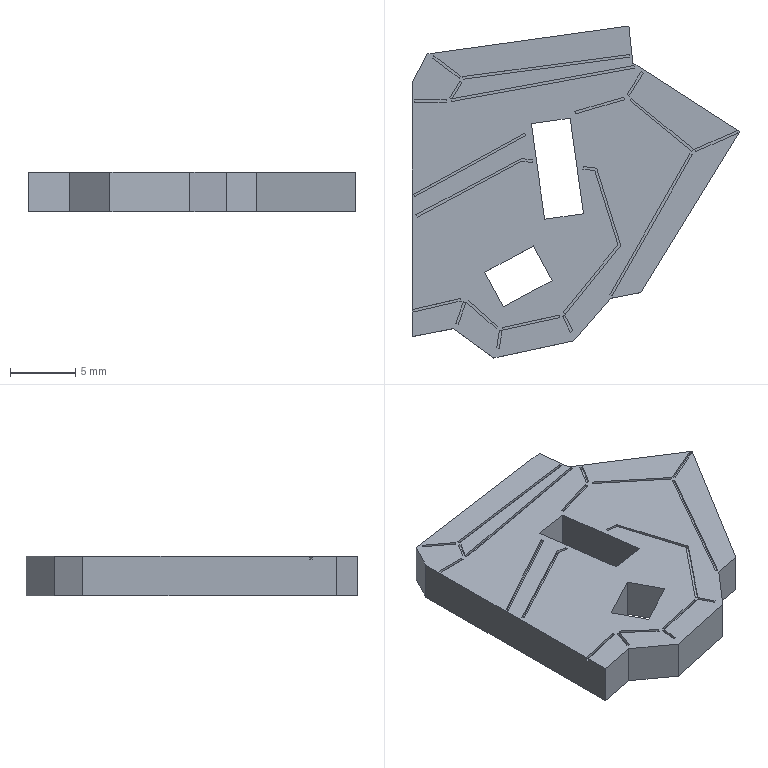Part | SolidWorks | features BaseBody 1 | 1 solid | 121 faces | box 25.081 x 25.399 x 3 mm | volume 1254 mm3 | plane 111 | spline 10